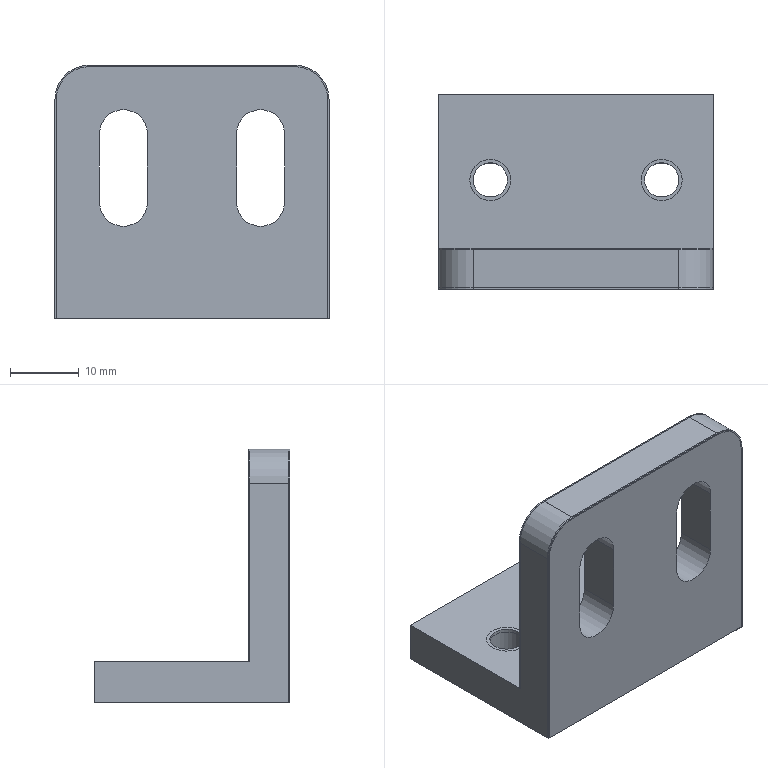Part | 2 solids | 52 faces | box 40 x 28.5 x 37 mm | volume 25348 mm3 | plane 30 | cylinder 16 | cone 6 | commonest cylinder face diameters 7 x8 5 x4 10 x4
STEP:
#1=CARTESIAN_POINT('',(37.,28.5,6.));
#2=VERTEX_POINT('',#1);
#3=CARTESIAN_POINT('',(-3.,28.5,6.));
#4=VERTEX_POINT('',#3);
#5=CARTESIAN_POINT('',(43.57,28.5,6.));
#6=DIRECTION('',(-1.,0.,0.));
#7=VECTOR('',#6,1000.);
#8=LINE('',#5,#7);
#9=EDGE_CURVE('',#2,#4,#8,.T.);
#10=ORIENTED_EDGE('',*,*,#9,.F.);
#11=CARTESIAN_POINT('',(37.,28.5,0.));
#12=VERTEX_POINT('',#11);
#13=CARTESIAN_POINT('',(37.,28.5,0.));
#14=DIRECTION('',(0.,0.,1.));
#15=VECTOR('',#14,1000.);
#16=LINE('',#13,#15);
#17=EDGE_CURVE('',#12,#2,#16,.T.);
#18=ORIENTED_EDGE('',*,*,#17,.F.);
#19=CARTESIAN_POINT('',(-3.,28.5,0.));
#20=VERTEX_POINT('',#19);
#21=CARTESIAN_POINT('',(18.5,28.5,0.));
#22=DIRECTION('',(-1.,0.,0.));
#23=VECTOR('',#22,1000.);
#24=LINE('',#21,#23);
#25=EDGE_CURVE('',#12,#20,#24,.T.);
#26=ORIENTED_EDGE('',*,*,#25,.T.);
#27=CARTESIAN_POINT('',(-3.,28.5,0.));
#28=DIRECTION('',(0.,0.,1.));
#29=VECTOR('',#28,1000.);
#30=LINE('',#27,#29);
#31=EDGE_CURVE('',#20,#4,#30,.T.);
#32=ORIENTED_EDGE('',*,*,#31,.T.);
#33=EDGE_LOOP('',(#10,#18,#26,#32));
#34=FACE_BOUND('',#33,.T.);
#35=CARTESIAN_POINT('',(18.5,28.5,0.));
#36=DIRECTION('',(0.,1.,0.));
#37=DIRECTION('',(0.,0.,1.));
#38=AXIS2_PLACEMENT_3D('',#35,#36,#37);
#39=PLANE('',#38);
#40=ADVANCED_FACE('',(#34),#39,.T.);
#41=CARTESIAN_POINT('',(2.,6.,37.));
#42=VERTEX_POINT('',#41);
#43=CARTESIAN_POINT('',(32.,6.,37.));
#44=VERTEX_POINT('',#43);
#45=CARTESIAN_POINT('',(43.57,6.,37.));
#46=DIRECTION('',(-1.,0.,0.));
#47=VECTOR('',#46,1000.);
#48=LINE('',#45,#47);
#49=EDGE_CURVE('',#42,#44,#48,.F.);
#50=ORIENTED_EDGE('',*,*,#49,.F.);
#51=CARTESIAN_POINT('',(2.,0.,37.));
#52=VERTEX_POINT('',#51);
#53=CARTESIAN_POINT('',(2.,14.25,37.));
#54=DIRECTION('',(0.,1.,0.));
#55=VECTOR('',#54,1000.);
#56=LINE('',#53,#55);
#57=EDGE_CURVE('',#42,#52,#56,.F.);
#58=ORIENTED_EDGE('',*,*,#57,.T.);
#59=CARTESIAN_POINT('',(32.,0.,37.));
#60=VERTEX_POINT('',#59);
#61=CARTESIAN_POINT('',(18.5,0.,37.));
#62=DIRECTION('',(-1.,0.,0.));
#63=VECTOR('',#62,1000.);
#64=LINE('',#61,#63);
#65=EDGE_CURVE('',#60,#52,#64,.T.);
#66=ORIENTED_EDGE('',*,*,#65,.F.);
#67=CARTESIAN_POINT('',(32.,14.25,37.));
#68=DIRECTION('',(0.,-1.,0.));
#69=VECTOR('',#68,1000.);
#70=LINE('',#67,#69);
#71=EDGE_CURVE('',#60,#44,#70,.F.);
#72=ORIENTED_EDGE('',*,*,#71,.T.);
#73=EDGE_LOOP('',(#50,#58,#66,#72));
#74=FACE_BOUND('',#73,.T.);
#75=CARTESIAN_POINT('',(18.5,14.25,37.));
#76=DIRECTION('',(0.,0.,1.));
#77=DIRECTION('',(1.,0.,0.));
#78=AXIS2_PLACEMENT_3D('',#75,#76,#77);
#79=PLANE('',#78);
#80=ADVANCED_FACE('',(#74),#79,.T.);
#81=CARTESIAN_POINT('',(10.5,0.,17.));
#82=VERTEX_POINT('',#81);
#83=CARTESIAN_POINT('',(10.5,0.,27.));
#84=VERTEX_POINT('',#83);
#85=CARTESIAN_POINT('',(10.5,0.,-0.5));
#86=DIRECTION('',(0.,0.,1.));
#87=VECTOR('',#86,1000.);
#88=LINE('',#85,#87);
#89=EDGE_CURVE('',#82,#84,#88,.T.);
#90=ORIENTED_EDGE('',*,*,#89,.F.);
#91=CARTESIAN_POINT('',(3.5,0.,17.));
#92=VERTEX_POINT('',#91);
#93=CARTESIAN_POINT('',(7.,0.,17.));
#94=DIRECTION('',(0.,-1.,0.));
#95=DIRECTION('',(0.,0.,-1.));
#96=AXIS2_PLACEMENT_3D('',#93,#94,#95);
#97=CIRCLE('',#96,3.5);
#98=EDGE_CURVE('',#92,#82,#97,.T.);
#99=ORIENTED_EDGE('',*,*,#98,.F.);
#100=CARTESIAN_POINT('',(3.5,0.,27.));
#101=VERTEX_POINT('',#100);
#102=CARTESIAN_POINT('',(3.5,0.,-0.5));
#103=DIRECTION('',(0.,0.,-1.));
#104=VECTOR('',#103,1000.);
#105=LINE('',#102,#104);
#106=EDGE_CURVE('',#101,#92,#105,.T.);
#107=ORIENTED_EDGE('',*,*,#106,.F.);
#108=CARTESIAN_POINT('',(7.,0.,27.));
#109=DIRECTION('',(0.,-1.,0.));
#110=DIRECTION('',(0.,0.,-1.));
#111=AXIS2_PLACEMENT_3D('',#108,#109,#110);
#112=CIRCLE('',#111,3.5);
#113=EDGE_CURVE('',#84,#101,#112,.T.);
#114=ORIENTED_EDGE('',*,*,#113,.F.);
#115=EDGE_LOOP('',(#90,#99,#107,#114));
#116=FACE_BOUND('',#115,.T.);
#117=CARTESIAN_POINT('',(30.5,0.,17.));
#118=VERTEX_POINT('',#117);
#119=CARTESIAN_POINT('',(30.5,0.,27.));
#120=VERTEX_POINT('',#119);
#121=CARTESIAN_POINT('',(30.5,0.,-0.5));
#122=DIRECTION('',(0.,0.,1.));
#123=VECTOR('',#122,1000.);
#124=LINE('',#121,#123);
#125=EDGE_CURVE('',#118,#120,#124,.T.);
#126=ORIENTED_EDGE('',*,*,#125,.F.);
#127=CARTESIAN_POINT('',(23.5,0.,17.));
#128=VERTEX_POINT('',#127);
#129=CARTESIAN_POINT('',(27.,0.,17.));
#130=DIRECTION('',(0.,-1.,0.));
#131=DIRECTION('',(0.,0.,-1.));
#132=AXIS2_PLACEMENT_3D('',#129,#130,#131);
#133=CIRCLE('',#132,3.5);
#134=EDGE_CURVE('',#128,#118,#133,.T.);
#135=ORIENTED_EDGE('',*,*,#134,.F.);
#136=CARTESIAN_POINT('',(23.5,0.,27.));
#137=VERTEX_POINT('',#136);
#138=CARTESIAN_POINT('',(23.5,0.,-0.5));
#139=DIRECTION('',(0.,0.,-1.));
#140=VECTOR('',#139,1000.);
#141=LINE('',#138,#140);
#142=EDGE_CURVE('',#137,#128,#141,.T.);
#143=ORIENTED_EDGE('',*,*,#142,.F.);
#144=CARTESIAN_POINT('',(27.,0.,27.));
#145=DIRECTION('',(0.,-1.,0.));
#146=DIRECTION('',(0.,0.,-1.));
#147=AXIS2_PLACEMENT_3D('',#144,#145,#146);
#148=CIRCLE('',#147,3.5);
#149=EDGE_CURVE('',#120,#137,#148,.T.);
#150=ORIENTED_EDGE('',*,*,#149,.F.);
#151=EDGE_LOOP('',(#126,#135,#143,#150));
#152=FACE_BOUND('',#151,.T.);
#153=ORIENTED_EDGE('',*,*,#65,.T.);
#154=CARTESIAN_POINT('',(-3.,0.,32.));
#155=VERTEX_POINT('',#154);
#156=CARTESIAN_POINT('',(2.,0.,32.));
#157=DIRECTION('',(0.,-1.,0.));
#158=DIRECTION('',(0.,0.,-1.));
#159=AXIS2_PLACEMENT_3D('',#156,#157,#158);
#160=CIRCLE('',#159,5.);
#161=EDGE_CURVE('',#52,#155,#160,.T.);
#162=ORIENTED_EDGE('',*,*,#161,.T.);
#163=CARTESIAN_POINT('',(-3.,0.,0.));
#164=VERTEX_POINT('',#163);
#165=CARTESIAN_POINT('',(-3.,0.,0.));
#166=DIRECTION('',(0.,0.,1.));
#167=VECTOR('',#166,1000.);
#168=LINE('',#165,#167);
#169=EDGE_CURVE('',#164,#155,#168,.T.);
#170=ORIENTED_EDGE('',*,*,#169,.F.);
#171=CARTESIAN_POINT('',(37.,0.,0.));
#172=VERTEX_POINT('',#171);
#173=CARTESIAN_POINT('',(18.5,0.,0.));
#174=DIRECTION('',(1.,0.,0.));
#175=VECTOR('',#174,1000.);
#176=LINE('',#173,#175);
#177=EDGE_CURVE('',#164,#172,#176,.T.);
#178=ORIENTED_EDGE('',*,*,#177,.T.);
#179=CARTESIAN_POINT('',(37.,0.,32.));
#180=VERTEX_POINT('',#179);
#181=CARTESIAN_POINT('',(37.,0.,0.));
#182=DIRECTION('',(0.,0.,1.));
#183=VECTOR('',#182,1000.);
#184=LINE('',#181,#183);
#185=EDGE_CURVE('',#172,#180,#184,.T.);
#186=ORIENTED_EDGE('',*,*,#185,.T.);
#187=CARTESIAN_POINT('',(32.,0.,32.));
#188=DIRECTION('',(0.,-1.,0.));
#189=DIRECTION('',(0.,0.,-1.));
#190=AXIS2_PLACEMENT_3D('',#187,#188,#189);
#191=CIRCLE('',#190,5.);
#192=EDGE_CURVE('',#180,#60,#191,.T.);
#193=ORIENTED_EDGE('',*,*,#192,.T.);
#194=EDGE_LOOP('',(#153,#162,#170,#178,#186,#193));
#195=FACE_BOUND('',#194,.T.);
#196=CARTESIAN_POINT('',(18.5,0.,0.));
#197=DIRECTION('',(0.,-1.,0.));
#198=DIRECTION('',(0.,0.,-1.));
#199=AXIS2_PLACEMENT_3D('',#196,#197,#198);
#200=PLANE('',#199);
#201=ADVANCED_FACE('',(#116,#152,#195),#200,.T.);
#202=ORIENTED_EDGE('',*,*,#169,.T.);
#203=CARTESIAN_POINT('',(-3.,6.,32.));
#204=VERTEX_POINT('',#203);
#205=CARTESIAN_POINT('',(-3.,14.25,32.));
#206=DIRECTION('',(0.,1.,0.));
#207=VECTOR('',#206,1000.);
#208=LINE('',#205,#207);
#209=EDGE_CURVE('',#155,#204,#208,.T.);
#210=ORIENTED_EDGE('',*,*,#209,.T.);
#211=CARTESIAN_POINT('',(-3.,6.,6.));
#212=VERTEX_POINT('',#211);
#213=CARTESIAN_POINT('',(-3.,6.,0.));
#214=DIRECTION('',(0.,0.,1.));
#215=VECTOR('',#214,1000.);
#216=LINE('',#213,#215);
#217=EDGE_CURVE('',#212,#204,#216,.T.);
#218=ORIENTED_EDGE('',*,*,#217,.F.);
#219=CARTESIAN_POINT('',(-3.,14.25,6.));
#220=DIRECTION('',(0.,-1.,0.));
#221=VECTOR('',#220,1000.);
#222=LINE('',#219,#221);
#223=EDGE_CURVE('',#4,#212,#222,.T.);
#224=ORIENTED_EDGE('',*,*,#223,.F.);
#225=ORIENTED_EDGE('',*,*,#31,.F.);
#226=CARTESIAN_POINT('',(-3.,14.25,0.));
#227=DIRECTION('',(0.,-1.,0.));
#228=VECTOR('',#227,1000.);
#229=LINE('',#226,#228);
#230=EDGE_CURVE('',#20,#164,#229,.T.);
#231=ORIENTED_EDGE('',*,*,#230,.T.);
#232=EDGE_LOOP('',(#202,#210,#218,#224,#225,#231));
#233=FACE_BOUND('',#232,.T.);
#234=CARTESIAN_POINT('',(-3.,14.25,0.));
#235=DIRECTION('',(-1.,0.,0.));
#236=DIRECTION('',(0.,0.,1.));
#237=AXIS2_PLACEMENT_3D('',#234,#235,#236);
#238=PLANE('',#237);
#239=ADVANCED_FACE('',(#233),#238,.T.);
#240=CARTESIAN_POINT('',(32.,16.,0.));
#241=VERTEX_POINT('',#240);
#242=CARTESIAN_POINT('',(29.5,16.,0.));
#243=DIRECTION('',(0.,0.,1.));
#244=DIRECTION('',(1.,0.,0.));
#245=AXIS2_PLACEMENT_3D('',#242,#243,#244);
#246=CIRCLE('',#245,2.5);
#247=EDGE_CURVE('',#241,#241,#246,.T.);
#248=ORIENTED_EDGE('',*,*,#247,.T.);
#249=EDGE_LOOP('',(#248));
#250=FACE_BOUND('',#249,.T.);
#251=CARTESIAN_POINT('',(7.,16.,0.));
#252=VERTEX_POINT('',#251);
#253=CARTESIAN_POINT('',(4.5,16.,0.));
#254=DIRECTION('',(0.,0.,1.));
#255=DIRECTION('',(1.,0.,0.));
#256=AXIS2_PLACEMENT_3D('',#253,#254,#255);
#257=CIRCLE('',#256,2.5);
#258=EDGE_CURVE('',#252,#252,#257,.T.);
#259=ORIENTED_EDGE('',*,*,#258,.T.);
#260=EDGE_LOOP('',(#259));
#261=FACE_BOUND('',#260,.T.);
#262=CARTESIAN_POINT('',(37.,14.25,0.));
#263=DIRECTION('',(0.,1.,0.));
#264=VECTOR('',#263,1000.);
#265=LINE('',#262,#264);
#266=EDGE_CURVE('',#172,#12,#265,.T.);
#267=ORIENTED_EDGE('',*,*,#266,.F.);
#268=ORIENTED_EDGE('',*,*,#177,.F.);
#269=ORIENTED_EDGE('',*,*,#230,.F.);
#270=ORIENTED_EDGE('',*,*,#25,.F.);
#271=EDGE_LOOP('',(#267,#268,#269,#270));
#272=FACE_BOUND('',#271,.T.);
#273=CARTESIAN_POINT('',(18.5,14.25,0.));
#274=DIRECTION('',(0.,0.,-1.));
#275=DIRECTION('',(-1.,0.,0.));
#276=AXIS2_PLACEMENT_3D('',#273,#274,#275);
#277=PLANE('',#276);
#278=ADVANCED_FACE('',(#250,#261,#272),#277,.T.);
#279=CARTESIAN_POINT('',(37.,6.,32.));
#280=VERTEX_POINT('',#279);
#281=CARTESIAN_POINT('',(37.,6.,6.));
#282=VERTEX_POINT('',#281);
#283=CARTESIAN_POINT('',(37.,6.,0.));
#284=DIRECTION('',(0.,0.,-1.));
#285=VECTOR('',#284,1000.);
#286=LINE('',#283,#285);
#287=EDGE_CURVE('',#280,#282,#286,.T.);
#288=ORIENTED_EDGE('',*,*,#287,.F.);
#289=CARTESIAN_POINT('',(37.,14.25,32.));
#290=DIRECTION('',(0.,-1.,0.));
#291=VECTOR('',#290,1000.);
#292=LINE('',#289,#291);
#293=EDGE_CURVE('',#280,#180,#292,.T.);
#294=ORIENTED_EDGE('',*,*,#293,.T.);
#295=ORIENTED_EDGE('',*,*,#185,.F.);
#296=ORIENTED_EDGE('',*,*,#266,.T.);
#297=ORIENTED_EDGE('',*,*,#17,.T.);
#298=CARTESIAN_POINT('',(37.,14.25,6.));
#299=DIRECTION('',(0.,1.,0.));
#300=VECTOR('',#299,1000.);
#301=LINE('',#298,#300);
#302=EDGE_CURVE('',#282,#2,#301,.T.);
#303=ORIENTED_EDGE('',*,*,#302,.F.);
#304=EDGE_LOOP('',(#288,#294,#295,#296,#297,#303));
#305=FACE_BOUND('',#304,.T.);
#306=CARTESIAN_POINT('',(37.,14.25,0.));
#307=DIRECTION('',(1.,0.,0.));
#308=DIRECTION('',(0.,0.,-1.));
#309=AXIS2_PLACEMENT_3D('',#306,#307,#308);
#310=PLANE('',#309);
#311=ADVANCED_FACE('',(#305),#310,.T.);
#312=CARTESIAN_POINT('',(27.,16.,6.));
#313=VERTEX_POINT('',#312);
#314=CARTESIAN_POINT('',(29.5,16.,6.));
#315=DIRECTION('',(0.,0.,-1.));
#316=DIRECTION('',(-1.,0.,0.));
#317=AXIS2_PLACEMENT_3D('',#314,#315,#316);
#318=CIRCLE('',#317,2.5);
#319=EDGE_CURVE('',#313,#313,#318,.T.);
#320=ORIENTED_EDGE('',*,*,#319,.T.);
#321=EDGE_LOOP('',(#320));
#322=FACE_BOUND('',#321,.T.);
#323=CARTESIAN_POINT('',(2.,16.,6.));
#324=VERTEX_POINT('',#323);
#325=CARTESIAN_POINT('',(4.5,16.,6.));
#326=DIRECTION('',(0.,0.,-1.));
#327=DIRECTION('',(-1.,0.,0.));
#328=AXIS2_PLACEMENT_3D('',#325,#326,#327);
#329=CIRCLE('',#328,2.5);
#330=EDGE_CURVE('',#324,#324,#329,.T.);
#331=ORIENTED_EDGE('',*,*,#330,.T.);
#332=EDGE_LOOP('',(#331));
#333=FACE_BOUND('',#332,.T.);
#334=ORIENTED_EDGE('',*,*,#223,.T.);
#335=CARTESIAN_POINT('',(43.57,6.,6.));
#336=DIRECTION('',(-1.,0.,0.));
#337=VECTOR('',#336,1000.);
#338=LINE('',#335,#337);
#339=EDGE_CURVE('',#212,#282,#338,.F.);
#340=ORIENTED_EDGE('',*,*,#339,.T.);
#341=ORIENTED_EDGE('',*,*,#302,.T.);
#342=ORIENTED_EDGE('',*,*,#9,.T.);
#343=EDGE_LOOP('',(#334,#340,#341,#342));
#344=FACE_BOUND('',#343,.T.);
#345=CARTESIAN_POINT('',(43.57,28.5,6.));
#346=DIRECTION('',(0.,0.,-1.));
#347=DIRECTION('',(-1.,0.,0.));
#348=AXIS2_PLACEMENT_3D('',#345,#346,#347);
#349=PLANE('',#348);
#350=ADVANCED_FACE('',(#322,#333,#344),#349,.F.);
#351=CARTESIAN_POINT('',(10.5,6.,17.));
#352=VERTEX_POINT('',#351);
#353=CARTESIAN_POINT('',(3.5,6.,17.));
#354=VERTEX_POINT('',#353);
#355=CARTESIAN_POINT('',(7.,6.,17.));
#356=DIRECTION('',(0.,1.,0.));
#357=DIRECTION('',(0.,0.,1.));
#358=AXIS2_PLACEMENT_3D('',#355,#356,#357);
#359=CIRCLE('',#358,3.5);
#360=EDGE_CURVE('',#352,#354,#359,.T.);
#361=ORIENTED_EDGE('',*,*,#360,.F.);
#362=CARTESIAN_POINT('',(10.5,6.,27.));
#363=VERTEX_POINT('',#362);
#364=CARTESIAN_POINT('',(10.5,6.,22.));
#365=DIRECTION('',(0.,0.,1.));
#366=VECTOR('',#365,1000.);
#367=LINE('',#364,#366);
#368=EDGE_CURVE('',#352,#363,#367,.T.);
#369=ORIENTED_EDGE('',*,*,#368,.T.);
#370=CARTESIAN_POINT('',(3.5,6.,27.));
#371=VERTEX_POINT('',#370);
#372=CARTESIAN_POINT('',(7.,6.,27.));
#373=DIRECTION('',(0.,1.,0.));
#374=DIRECTION('',(0.,0.,1.));
#375=AXIS2_PLACEMENT_3D('',#372,#373,#374);
#376=CIRCLE('',#375,3.5);
#377=EDGE_CURVE('',#371,#363,#376,.T.);
#378=ORIENTED_EDGE('',*,*,#377,.F.);
#379=CARTESIAN_POINT('',(3.5,6.,22.));
#380=DIRECTION('',(0.,0.,1.));
#381=VECTOR('',#380,1000.);
#382=LINE('',#379,#381);
#383=EDGE_CURVE('',#354,#371,#382,.T.);
#384=ORIENTED_EDGE('',*,*,#383,.F.);
#385=EDGE_LOOP('',(#361,#369,#378,#384));
#386=FACE_BOUND('',#385,.T.);
#387=CARTESIAN_POINT('',(30.5,6.,17.));
#388=VERTEX_POINT('',#387);
#389=CARTESIAN_POINT('',(23.5,6.,17.));
#390=VERTEX_POINT('',#389);
#391=CARTESIAN_POINT('',(27.,6.,17.));
#392=DIRECTION('',(0.,1.,0.));
#393=DIRECTION('',(0.,0.,1.));
#394=AXIS2_PLACEMENT_3D('',#391,#392,#393);
#395=CIRCLE('',#394,3.5);
#396=EDGE_CURVE('',#388,#390,#395,.T.);
#397=ORIENTED_EDGE('',*,*,#396,.F.);
#398=CARTESIAN_POINT('',(30.5,6.,27.));
#399=VERTEX_POINT('',#398);
#400=CARTESIAN_POINT('',(30.5,6.,22.));
#401=DIRECTION('',(0.,0.,1.));
#402=VECTOR('',#401,1000.);
#403=LINE('',#400,#402);
#404=EDGE_CURVE('',#388,#399,#403,.T.);
#405=ORIENTED_EDGE('',*,*,#404,.T.);
#406=CARTESIAN_POINT('',(23.5,6.,27.));
#407=VERTEX_POINT('',#406);
#408=CARTESIAN_POINT('',(27.,6.,27.));
#409=DIRECTION('',(0.,1.,0.));
#410=DIRECTION('',(0.,0.,1.));
#411=AXIS2_PLACEMENT_3D('',#408,#409,#410);
#412=CIRCLE('',#411,3.5);
#413=EDGE_CURVE('',#407,#399,#412,.T.);
#414=ORIENTED_EDGE('',*,*,#413,.F.);
#415=CARTESIAN_POINT('',(23.5,6.,22.));
#416=DIRECTION('',(0.,0.,1.));
#417=VECTOR('',#416,1000.);
#418=LINE('',#415,#417);
#419=EDGE_CURVE('',#390,#407,#418,.T.);
#420=ORIENTED_EDGE('',*,*,#419,.F.);
#421=EDGE_LOOP('',(#397,#405,#414,#420));
#422=FACE_BOUND('',#421,.T.);
#423=ORIENTED_EDGE('',*,*,#217,.T.);
#424=CARTESIAN_POINT('',(2.,6.,32.));
#425=DIRECTION('',(0.,-1.,0.));
#426=DIRECTION('',(0.,0.,-1.));
#427=AXIS2_PLACEMENT_3D('',#424,#425,#426);
#428=CIRCLE('',#427,5.);
#429=EDGE_CURVE('',#204,#42,#428,.F.);
#430=ORIENTED_EDGE('',*,*,#429,.T.);
#431=ORIENTED_EDGE('',*,*,#49,.T.);
#432=CARTESIAN_POINT('',(32.,6.,32.));
#433=DIRECTION('',(0.,-1.,0.));
#434=DIRECTION('',(0.,0.,-1.));
#435=AXIS2_PLACEMENT_3D('',#432,#433,#434);
#436=CIRCLE('',#435,5.);
#437=EDGE_CURVE('',#44,#280,#436,.F.);
#438=ORIENTED_EDGE('',*,*,#437,.T.);
#439=ORIENTED_EDGE('',*,*,#287,.T.);
#440=ORIENTED_EDGE('',*,*,#339,.F.);
#441=EDGE_LOOP('',(#423,#430,#431,#438,#439,#440));
#442=FACE_BOUND('',#441,.T.);
#443=CARTESIAN_POINT('',(43.57,6.,37.));
#444=DIRECTION('',(0.,-1.,0.));
#445=DIRECTION('',(0.,0.,-1.));
#446=AXIS2_PLACEMENT_3D('',#443,#444,#445);
#447=PLANE('',#446);
#448=ADVANCED_FACE('',(#386,#422,#442),#447,.F.);
#449=ORIENTED_EDGE('',*,*,#125,.T.);
#450=CARTESIAN_POINT('',(30.5,6.,27.));
#451=DIRECTION('',(0.,1.,0.));
#452=VECTOR('',#451,1000.);
#453=LINE('',#450,#452);
#454=EDGE_CURVE('',#399,#120,#453,.F.);
#455=ORIENTED_EDGE('',*,*,#454,.F.);
#456=ORIENTED_EDGE('',*,*,#404,.F.);
#457=CARTESIAN_POINT('',(30.5,6.,17.));
#458=DIRECTION('',(0.,1.,0.));
#459=VECTOR('',#458,1000.);
#460=LINE('',#457,#459);
#461=EDGE_CURVE('',#388,#118,#460,.F.);
#462=ORIENTED_EDGE('',*,*,#461,.T.);
#463=EDGE_LOOP('',(#449,#455,#456,#462));
#464=FACE_BOUND('',#463,.T.);
#465=CARTESIAN_POINT('',(30.5,6.,22.));
#466=DIRECTION('',(1.,0.,0.));
#467=DIRECTION('',(0.,0.,-1.));
#468=AXIS2_PLACEMENT_3D('',#465,#466,#467);
#469=PLANE('',#468);
#470=ADVANCED_FACE('',(#464),#469,.F.);
#471=ORIENTED_EDGE('',*,*,#134,.T.);
#472=ORIENTED_EDGE('',*,*,#461,.F.);
#473=ORIENTED_EDGE('',*,*,#396,.T.);
#474=CARTESIAN_POINT('',(23.5,6.,17.));
#475=DIRECTION('',(0.,1.,0.));
#476=VECTOR('',#475,1000.);
#477=LINE('',#474,#476);
#478=EDGE_CURVE('',#390,#128,#477,.F.);
#479=ORIENTED_EDGE('',*,*,#478,.T.);
#480=EDGE_LOOP('',(#471,#472,#473,#479));
#481=FACE_BOUND('',#480,.T.);
#482=CARTESIAN_POINT('',(27.,6.,17.));
#483=DIRECTION('',(0.,1.,0.));
#484=DIRECTION('',(0.,0.,1.));
#485=AXIS2_PLACEMENT_3D('',#482,#483,#484);
#486=CYLINDRICAL_SURFACE('',#485,3.5);
#487=ADVANCED_FACE('',(#481),#486,.F.);
#488=ORIENTED_EDGE('',*,*,#142,.T.);
#489=ORIENTED_EDGE('',*,*,#478,.F.);
#490=ORIENTED_EDGE('',*,*,#419,.T.);
#491=CARTESIAN_POINT('',(23.5,6.,27.));
#492=DIRECTION('',(0.,1.,0.));
#493=VECTOR('',#492,1000.);
#494=LINE('',#491,#493);
#495=EDGE_CURVE('',#407,#137,#494,.F.);
#496=ORIENTED_EDGE('',*,*,#495,.T.);
#497=EDGE_LOOP('',(#488,#489,#490,#496));
#498=FACE_BOUND('',#497,.T.);
#499=CARTESIAN_POINT('',(23.5,6.,22.));
#500=DIRECTION('',(-1.,0.,0.));
#501=DIRECTION('',(0.,0.,1.));
#502=AXIS2_PLACEMENT_3D('',#499,#500,#501);
#503=PLANE('',#502);
#504=ADVANCED_FACE('',(#498),#503,.F.);
#505=ORIENTED_EDGE('',*,*,#149,.T.);
#506=ORIENTED_EDGE('',*,*,#495,.F.);
#507=ORIENTED_EDGE('',*,*,#413,.T.);
#508=ORIENTED_EDGE('',*,*,#454,.T.);
#509=EDGE_LOOP('',(#505,#506,#507,#508));
#510=FACE_BOUND('',#509,.T.);
#511=CARTESIAN_POINT('',(27.,6.,27.));
#512=DIRECTION('',(0.,1.,0.));
#513=DIRECTION('',(0.,0.,1.));
#514=AXIS2_PLACEMENT_3D('',#511,#512,#513);
#515=CYLINDRICAL_SURFACE('',#514,3.5);
#516=ADVANCED_FACE('',(#510),#515,.F.);
#517=ORIENTED_EDGE('',*,*,#89,.T.);
#518=CARTESIAN_POINT('',(10.5,6.,27.));
#519=DIRECTION('',(0.,1.,0.));
#520=VECTOR('',#519,1000.);
#521=LINE('',#518,#520);
#522=EDGE_CURVE('',#84,#363,#521,.T.);
#523=ORIENTED_EDGE('',*,*,#522,.T.);
#524=ORIENTED_EDGE('',*,*,#368,.F.);
#525=CARTESIAN_POINT('',(10.5,6.,17.));
#526=DIRECTION('',(0.,1.,0.));
#527=VECTOR('',#526,1000.);
#528=LINE('',#525,#527);
#529=EDGE_CURVE('',#82,#352,#528,.T.);
#530=ORIENTED_EDGE('',*,*,#529,.F.);
#531=EDGE_LOOP('',(#517,#523,#524,#530));
#532=FACE_BOUND('',#531,.T.);
#533=CARTESIAN_POINT('',(10.5,6.,22.));
#534=DIRECTION('',(1.,0.,0.));
#535=DIRECTION('',(0.,0.,-1.));
#536=AXIS2_PLACEMENT_3D('',#533,#534,#535);
#537=PLANE('',#536);
#538=ADVANCED_FACE('',(#532),#537,.F.);
#539=ORIENTED_EDGE('',*,*,#98,.T.);
#540=ORIENTED_EDGE('',*,*,#529,.T.);
#541=ORIENTED_EDGE('',*,*,#360,.T.);
#542=CARTESIAN_POINT('',(3.5,6.,17.));
#543=DIRECTION('',(0.,1.,0.));
#544=VECTOR('',#543,1000.);
#545=LINE('',#542,#544);
#546=EDGE_CURVE('',#92,#354,#545,.T.);
#547=ORIENTED_EDGE('',*,*,#546,.F.);
#548=EDGE_LOOP('',(#539,#540,#541,#547));
#549=FACE_BOUND('',#548,.T.);
#550=CARTESIAN_POINT('',(7.,6.,17.));
#551=DIRECTION('',(0.,1.,0.));
#552=DIRECTION('',(0.,0.,1.));
#553=AXIS2_PLACEMENT_3D('',#550,#551,#552);
#554=CYLINDRICAL_SURFACE('',#553,3.5);
#555=ADVANCED_FACE('',(#549),#554,.F.);
#556=ORIENTED_EDGE('',*,*,#106,.T.);
#557=ORIENTED_EDGE('',*,*,#546,.T.);
#558=ORIENTED_EDGE('',*,*,#383,.T.);
#559=CARTESIAN_POINT('',(3.5,6.,27.));
#560=DIRECTION('',(0.,1.,0.));
#561=VECTOR('',#560,1000.);
#562=LINE('',#559,#561);
#563=EDGE_CURVE('',#101,#371,#562,.T.);
#564=ORIENTED_EDGE('',*,*,#563,.F.);
#565=EDGE_LOOP('',(#556,#557,#558,#564));
#566=FACE_BOUND('',#565,.T.);
#567=CARTESIAN_POINT('',(3.5,6.,22.));
#568=DIRECTION('',(-1.,0.,0.));
#569=DIRECTION('',(0.,0.,1.));
#570=AXIS2_PLACEMENT_3D('',#567,#568,#569);
#571=PLANE('',#570);
#572=ADVANCED_FACE('',(#566),#571,.F.);
#573=ORIENTED_EDGE('',*,*,#113,.T.);
#574=ORIENTED_EDGE('',*,*,#563,.T.);
#575=ORIENTED_EDGE('',*,*,#377,.T.);
#576=ORIENTED_EDGE('',*,*,#522,.F.);
#577=EDGE_LOOP('',(#573,#574,#575,#576));
#578=FACE_BOUND('',#577,.T.);
#579=CARTESIAN_POINT('',(7.,6.,27.));
#580=DIRECTION('',(0.,1.,0.));
#581=DIRECTION('',(0.,0.,1.));
#582=AXIS2_PLACEMENT_3D('',#579,#580,#581);
#583=CYLINDRICAL_SURFACE('',#582,3.5);
#584=ADVANCED_FACE('',(#578),#583,.F.);
#585=ORIENTED_EDGE('',*,*,#161,.F.);
#586=ORIENTED_EDGE('',*,*,#57,.F.);
#587=ORIENTED_EDGE('',*,*,#429,.F.);
#588=ORIENTED_EDGE('',*,*,#209,.F.);
#589=EDGE_LOOP('',(#585,#586,#587,#588));
#590=FACE_BOUND('',#589,.T.);
#591=CARTESIAN_POINT('',(2.,14.25,32.));
#592=DIRECTION('',(0.,1.,0.));
#593=DIRECTION('',(0.,0.,1.));
#594=AXIS2_PLACEMENT_3D('',#591,#592,#593);
#595=CYLINDRICAL_SURFACE('',#594,5.);
#596=ADVANCED_FACE('',(#590),#595,.T.);
#597=ORIENTED_EDGE('',*,*,#437,.F.);
#598=ORIENTED_EDGE('',*,*,#71,.F.);
#599=ORIENTED_EDGE('',*,*,#192,.F.);
#600=ORIENTED_EDGE('',*,*,#293,.F.);
#601=EDGE_LOOP('',(#597,#598,#599,#600));
#602=FACE_BOUND('',#601,.T.);
#603=CARTESIAN_POINT('',(32.,14.25,32.));
#604=DIRECTION('',(0.,-1.,0.));
#605=DIRECTION('',(0.,0.,-1.));
#606=AXIS2_PLACEMENT_3D('',#603,#604,#605);
#607=CYLINDRICAL_SURFACE('',#606,5.);
#608=ADVANCED_FACE('',(#602),#607,.T.);
#609=ORIENTED_EDGE('',*,*,#258,.F.);
#610=EDGE_LOOP('',(#609));
#611=FACE_BOUND('',#610,.T.);
#612=ORIENTED_EDGE('',*,*,#330,.F.);
#613=EDGE_LOOP('',(#612));
#614=FACE_BOUND('',#613,.T.);
#615=CARTESIAN_POINT('',(4.5,16.,0.));
#616=DIRECTION('',(0.,0.,1.));
#617=DIRECTION('',(1.,0.,0.));
#618=AXIS2_PLACEMENT_3D('',#615,#616,#617);
#619=CYLINDRICAL_SURFACE('',#618,2.5);
#620=ADVANCED_FACE('',(#611,#614),#619,.F.);
#621=ORIENTED_EDGE('',*,*,#247,.F.);
#622=EDGE_LOOP('',(#621));
#623=FACE_BOUND('',#622,.T.);
#624=ORIENTED_EDGE('',*,*,#319,.F.);
#625=EDGE_LOOP('',(#624));
#626=FACE_BOUND('',#625,.T.);
#627=CARTESIAN_POINT('',(29.5,16.,0.));
#628=DIRECTION('',(0.,0.,1.));
#629=DIRECTION('',(1.,0.,0.));
#630=AXIS2_PLACEMENT_3D('',#627,#628,#629);
#631=CYLINDRICAL_SURFACE('',#630,2.5);
#632=ADVANCED_FACE('',(#623,#626),#631,.F.);
#633=CLOSED_SHELL('',(#40,#80,#201,#239,#278,#311,#350,#448,#470,#487,#504,#516,#538,#555,#572,#584,#596,#608,#620,#632));
#634=MANIFOLD_SOLID_BREP('',#633);
#635=CARTESIAN_POINT('',(37.,28.5,6.));
#636=VERTEX_POINT('',#635);
#637=CARTESIAN_POINT('',(-3.,28.5,6.));
#638=VERTEX_POINT('',#637);
#639=CARTESIAN_POINT('',(43.57,28.5,6.));
#640=DIRECTION('',(-1.,0.,0.));
#641=VECTOR('',#640,1000.);
#642=LINE('',#639,#641);
#643=EDGE_CURVE('',#636,#638,#642,.T.);
#644=ORIENTED_EDGE('',*,*,#643,.F.);
#645=CARTESIAN_POINT('',(37.,28.5,0.));
#646=VERTEX_POINT('',#645);
#647=CARTESIAN_POINT('',(37.,28.5,0.));
#648=DIRECTION('',(0.,0.,1.));
#649=VECTOR('',#648,1000.);
#650=LINE('',#647,#649);
#651=EDGE_CURVE('',#646,#636,#650,.T.);
#652=ORIENTED_EDGE('',*,*,#651,.F.);
#653=CARTESIAN_POINT('',(-3.,28.5,0.));
#654=VERTEX_POINT('',#653);
#655=CARTESIAN_POINT('',(18.5,28.5,0.));
#656=DIRECTION('',(-1.,0.,0.));
#657=VECTOR('',#656,1000.);
#658=LINE('',#655,#657);
#659=EDGE_CURVE('',#646,#654,#658,.T.);
#660=ORIENTED_EDGE('',*,*,#659,.T.);
#661=CARTESIAN_POINT('',(-3.,28.5,0.));
#662=DIRECTION('',(0.,0.,1.));
#663=VECTOR('',#662,1000.);
#664=LINE('',#661,#663);
#665=EDGE_CURVE('',#654,#638,#664,.T.);
#666=ORIENTED_EDGE('',*,*,#665,.T.);
#667=EDGE_LOOP('',(#644,#652,#660,#666));
#668=FACE_BOUND('',#667,.T.);
#669=CARTESIAN_POINT('',(18.5,28.5,0.));
#670=DIRECTION('',(0.,1.,0.));
#671=DIRECTION('',(0.,0.,1.));
#672=AXIS2_PLACEMENT_3D('',#669,#670,#671);
#673=PLANE('',#672);
#674=ADVANCED_FACE('',(#668),#673,.T.);
#675=CARTESIAN_POINT('',(2.,5.8,37.));
#676=VERTEX_POINT('',#675);
#677=CARTESIAN_POINT('',(2.,0.2,37.));
#678=VERTEX_POINT('',#677);
#679=CARTESIAN_POINT('',(2.,14.25,37.));
#680=DIRECTION('',(0.,1.,0.));
#681=VECTOR('',#680,1000.);
#682=LINE('',#679,#681);
#683=EDGE_CURVE('',#676,#678,#682,.F.);
#684=ORIENTED_EDGE('',*,*,#683,.T.);
#685=CARTESIAN_POINT('',(32.,0.2,37.));
#686=VERTEX_POINT('',#685);
#687=CARTESIAN_POINT('',(18.5,0.2,37.));
#688=DIRECTION('',(1.,0.,0.));
#689=VECTOR('',#688,1000.);
#690=LINE('',#687,#689);
#691=EDGE_CURVE('',#678,#686,#690,.T.);
#692=ORIENTED_EDGE('',*,*,#691,.T.);
#693=CARTESIAN_POINT('',(32.,5.8,37.));
#694=VERTEX_POINT('',#693);
#695=CARTESIAN_POINT('',(32.,14.25,37.));
#696=DIRECTION('',(0.,-1.,0.));
#697=VECTOR('',#696,1000.);
#698=LINE('',#695,#697);
#699=EDGE_CURVE('',#686,#694,#698,.F.);
#700=ORIENTED_EDGE('',*,*,#699,.T.);
#701=CARTESIAN_POINT('',(2.,5.8,37.));
#702=DIRECTION('',(-1.,0.,0.));
#703=VECTOR('',#702,1000.);
#704=LINE('',#701,#703);
#705=EDGE_CURVE('',#694,#676,#704,.T.);
#706=ORIENTED_EDGE('',*,*,#705,.T.);
#707=EDGE_LOOP('',(#684,#692,#700,#706));
#708=FACE_BOUND('',#707,.T.);
#709=CARTESIAN_POINT('',(18.5,14.25,37.));
#710=DIRECTION('',(0.,0.,1.));
#711=DIRECTION('',(1.,0.,0.));
#712=AXIS2_PLACEMENT_3D('',#709,#710,#711);
#713=PLANE('',#712);
#714=ADVANCED_FACE('',(#708),#713,.T.);
#715=CARTESIAN_POINT('',(10.5,0.,17.));
#716=VERTEX_POINT('',#715);
#717=CARTESIAN_POINT('',(10.5,0.,27.));
#718=VERTEX_POINT('',#717);
#719=CARTESIAN_POINT('',(10.5,0.,-0.5));
#720=DIRECTION('',(0.,0.,1.));
#721=VECTOR('',#720,1000.);
#722=LINE('',#719,#721);
#723=EDGE_CURVE('',#716,#718,#722,.T.);
#724=ORIENTED_EDGE('',*,*,#723,.F.);
#725=CARTESIAN_POINT('',(3.5,0.,17.));
#726=VERTEX_POINT('',#725);
#727=CARTESIAN_POINT('',(7.,0.,17.));
#728=DIRECTION('',(0.,-1.,0.));
#729=DIRECTION('',(0.,0.,-1.));
#730=AXIS2_PLACEMENT_3D('',#727,#728,#729);
#731=CIRCLE('',#730,3.5);
#732=EDGE_CURVE('',#726,#716,#731,.T.);
#733=ORIENTED_EDGE('',*,*,#732,.F.);
#734=CARTESIAN_POINT('',(3.5,0.,27.));
#735=VERTEX_POINT('',#734);
#736=CARTESIAN_POINT('',(3.5,0.,-0.5));
#737=DIRECTION('',(0.,0.,-1.));
#738=VECTOR('',#737,1000.);
#739=LINE('',#736,#738);
#740=EDGE_CURVE('',#735,#726,#739,.T.);
#741=ORIENTED_EDGE('',*,*,#740,.F.);
#742=CARTESIAN_POINT('',(7.,0.,27.));
#743=DIRECTION('',(0.,-1.,0.));
#744=DIRECTION('',(0.,0.,-1.));
#745=AXIS2_PLACEMENT_3D('',#742,#743,#744);
#746=CIRCLE('',#745,3.5);
#747=EDGE_CURVE('',#718,#735,#746,.T.);
#748=ORIENTED_EDGE('',*,*,#747,.F.);
#749=EDGE_LOOP('',(#724,#733,#741,#748));
#750=FACE_BOUND('',#749,.T.);
#751=CARTESIAN_POINT('',(30.5,0.,17.));
#752=VERTEX_POINT('',#751);
#753=CARTESIAN_POINT('',(30.5,0.,27.));
#754=VERTEX_POINT('',#753);
#755=CARTESIAN_POINT('',(30.5,0.,-0.5));
#756=DIRECTION('',(0.,0.,1.));
#757=VECTOR('',#756,1000.);
#758=LINE('',#755,#757);
#759=EDGE_CURVE('',#752,#754,#758,.T.);
#760=ORIENTED_EDGE('',*,*,#759,.F.);
#761=CARTESIAN_POINT('',(23.5,0.,17.));
#762=VERTEX_POINT('',#761);
#763=CARTESIAN_POINT('',(27.,0.,17.));
#764=DIRECTION('',(0.,-1.,0.));
#765=DIRECTION('',(0.,0.,-1.));
#766=AXIS2_PLACEMENT_3D('',#763,#764,#765);
#767=CIRCLE('',#766,3.5);
#768=EDGE_CURVE('',#762,#752,#767,.T.);
#769=ORIENTED_EDGE('',*,*,#768,.F.);
#770=CARTESIAN_POINT('',(23.5,0.,27.));
#771=VERTEX_POINT('',#770);
#772=CARTESIAN_POINT('',(23.5,0.,-0.5));
#773=DIRECTION('',(0.,0.,-1.));
#774=VECTOR('',#773,1000.);
#775=LINE('',#772,#774);
#776=EDGE_CURVE('',#771,#762,#775,.T.);
#777=ORIENTED_EDGE('',*,*,#776,.F.);
#778=CARTESIAN_POINT('',(27.,0.,27.));
#779=DIRECTION('',(0.,-1.,0.));
#780=DIRECTION('',(0.,0.,-1.));
#781=AXIS2_PLACEMENT_3D('',#778,#779,#780);
#782=CIRCLE('',#781,3.5);
#783=EDGE_CURVE('',#754,#771,#782,.T.);
#784=ORIENTED_EDGE('',*,*,#783,.F.);
#785=EDGE_LOOP('',(#760,#769,#777,#784));
#786=FACE_BOUND('',#785,.T.);
#787=CARTESIAN_POINT('',(-2.8,0.,0.));
#788=VERTEX_POINT('',#787);
#789=CARTESIAN_POINT('',(36.8,0.,0.));
#790=VERTEX_POINT('',#789);
#791=CARTESIAN_POINT('',(18.5,0.,0.));
#792=DIRECTION('',(1.,0.,0.));
#793=VECTOR('',#792,1000.);
#794=LINE('',#791,#793);
#795=EDGE_CURVE('',#788,#790,#794,.T.);
#796=ORIENTED_EDGE('',*,*,#795,.T.);
#797=CARTESIAN_POINT('',(36.8,0.,32.));
#798=VERTEX_POINT('',#797);
#799=CARTESIAN_POINT('',(36.8,0.,0.));
#800=DIRECTION('',(0.,0.,1.));
#801=VECTOR('',#800,1000.);
#802=LINE('',#799,#801);
#803=EDGE_CURVE('',#790,#798,#802,.T.);
#804=ORIENTED_EDGE('',*,*,#803,.T.);
#805=CARTESIAN_POINT('',(32.,0.,36.8));
#806=VERTEX_POINT('',#805);
#807=CARTESIAN_POINT('',(32.,0.,32.));
#808=DIRECTION('',(0.,-1.,0.));
#809=DIRECTION('',(0.,0.,-1.));
#810=AXIS2_PLACEMENT_3D('',#807,#808,#809);
#811=CIRCLE('',#810,4.8);
#812=EDGE_CURVE('',#798,#806,#811,.T.);
#813=ORIENTED_EDGE('',*,*,#812,.T.);
#814=CARTESIAN_POINT('',(2.,0.,36.8));
#815=VERTEX_POINT('',#814);
#816=CARTESIAN_POINT('',(18.5,0.,36.8));
#817=DIRECTION('',(-1.,0.,0.));
#818=VECTOR('',#817,1000.);
#819=LINE('',#816,#818);
#820=EDGE_CURVE('',#806,#815,#819,.T.);
#821=ORIENTED_EDGE('',*,*,#820,.T.);
#822=CARTESIAN_POINT('',(-2.8,0.,32.));
#823=VERTEX_POINT('',#822);
#824=CARTESIAN_POINT('',(2.,0.,32.));
#825=DIRECTION('',(0.,-1.,0.));
#826=DIRECTION('',(0.,0.,-1.));
#827=AXIS2_PLACEMENT_3D('',#824,#825,#826);
#828=CIRCLE('',#827,4.8);
#829=EDGE_CURVE('',#815,#823,#828,.T.);
#830=ORIENTED_EDGE('',*,*,#829,.T.);
#831=CARTESIAN_POINT('',(-2.8,0.,0.));
#832=DIRECTION('',(0.,0.,-1.));
#833=VECTOR('',#832,1000.);
#834=LINE('',#831,#833);
#835=EDGE_CURVE('',#823,#788,#834,.T.);
#836=ORIENTED_EDGE('',*,*,#835,.T.);
#837=EDGE_LOOP('',(#796,#804,#813,#821,#830,#836));
#838=FACE_BOUND('',#837,.T.);
#839=CARTESIAN_POINT('',(18.5,0.,0.));
#840=DIRECTION('',(0.,-1.,0.));
#841=DIRECTION('',(0.,0.,-1.));
#842=AXIS2_PLACEMENT_3D('',#839,#840,#841);
#843=PLANE('',#842);
#844=ADVANCED_FACE('',(#750,#786,#838),#843,.T.);
#845=CARTESIAN_POINT('',(-3.,0.2,0.));
#846=VERTEX_POINT('',#845);
#847=CARTESIAN_POINT('',(-3.,14.25,0.));
#848=DIRECTION('',(0.,-1.,0.));
#849=VECTOR('',#848,1000.);
#850=LINE('',#847,#849);
#851=EDGE_CURVE('',#654,#846,#850,.T.);
#852=ORIENTED_EDGE('',*,*,#851,.T.);
#853=CARTESIAN_POINT('',(-3.,0.2,32.));
#854=VERTEX_POINT('',#853);
#855=CARTESIAN_POINT('',(-3.,0.2,0.));
#856=DIRECTION('',(0.,0.,1.));
#857=VECTOR('',#856,1000.);
#858=LINE('',#855,#857);
#859=EDGE_CURVE('',#846,#854,#858,.T.);
#860=ORIENTED_EDGE('',*,*,#859,.T.);
#861=CARTESIAN_POINT('',(-3.,5.8,32.));
#862=VERTEX_POINT('',#861);
#863=CARTESIAN_POINT('',(-3.,14.25,32.));
#864=DIRECTION('',(0.,1.,0.));
#865=VECTOR('',#864,1000.);
#866=LINE('',#863,#865);
#867=EDGE_CURVE('',#854,#862,#866,.T.);
#868=ORIENTED_EDGE('',*,*,#867,.T.);
#869=CARTESIAN_POINT('',(-3.,5.8,6.));
#870=VERTEX_POINT('',#869);
#871=CARTESIAN_POINT('',(-3.,5.8,6.));
#872=DIRECTION('',(0.,0.,-1.));
#873=VECTOR('',#872,1000.);
#874=LINE('',#871,#873);
#875=EDGE_CURVE('',#862,#870,#874,.T.);
#876=ORIENTED_EDGE('',*,*,#875,.T.);
#877=CARTESIAN_POINT('',(-3.,14.25,6.));
#878=DIRECTION('',(0.,-1.,0.));
#879=VECTOR('',#878,1000.);
#880=LINE('',#877,#879);
#881=EDGE_CURVE('',#638,#870,#880,.T.);
#882=ORIENTED_EDGE('',*,*,#881,.F.);
#883=ORIENTED_EDGE('',*,*,#665,.F.);
#884=EDGE_LOOP('',(#852,#860,#868,#876,#882,#883));
#885=FACE_BOUND('',#884,.T.);
#886=CARTESIAN_POINT('',(-3.,14.25,0.));
#887=DIRECTION('',(-1.,0.,0.));
#888=DIRECTION('',(0.,0.,1.));
#889=AXIS2_PLACEMENT_3D('',#886,#887,#888);
#890=PLANE('',#889);
#891=ADVANCED_FACE('',(#885),#890,.T.);
#892=CARTESIAN_POINT('',(32.,16.,0.));
#893=VERTEX_POINT('',#892);
#894=CARTESIAN_POINT('',(29.5,16.,0.));
#895=DIRECTION('',(0.,0.,1.));
#896=DIRECTION('',(1.,0.,0.));
#897=AXIS2_PLACEMENT_3D('',#894,#895,#896);
#898=CIRCLE('',#897,2.5);
#899=EDGE_CURVE('',#893,#893,#898,.T.);
#900=ORIENTED_EDGE('',*,*,#899,.T.);
#901=EDGE_LOOP('',(#900));
#902=FACE_BOUND('',#901,.T.);
#903=CARTESIAN_POINT('',(7.,16.,0.));
#904=VERTEX_POINT('',#903);
#905=CARTESIAN_POINT('',(4.5,16.,0.));
#906=DIRECTION('',(0.,0.,1.));
#907=DIRECTION('',(1.,0.,0.));
#908=AXIS2_PLACEMENT_3D('',#905,#906,#907);
#909=CIRCLE('',#908,2.5);
#910=EDGE_CURVE('',#904,#904,#909,.T.);
#911=ORIENTED_EDGE('',*,*,#910,.T.);
#912=EDGE_LOOP('',(#911));
#913=FACE_BOUND('',#912,.T.);
#914=CARTESIAN_POINT('',(37.,0.2,0.));
#915=VERTEX_POINT('',#914);
#916=CARTESIAN_POINT('',(37.,14.25,0.));
#917=DIRECTION('',(0.,1.,0.));
#918=VECTOR('',#917,1000.);
#919=LINE('',#916,#918);
#920=EDGE_CURVE('',#915,#646,#919,.T.);
#921=ORIENTED_EDGE('',*,*,#920,.F.);
#922=CARTESIAN_POINT('',(34.775,-2.025,0.));
#923=DIRECTION('',(0.7071,0.7071,0.));
#924=VECTOR('',#923,1000.);
#925=LINE('',#922,#924);
#926=EDGE_CURVE('',#915,#790,#925,.F.);
#927=ORIENTED_EDGE('',*,*,#926,.T.);
#928=ORIENTED_EDGE('',*,*,#795,.F.);
#929=CARTESIAN_POINT('',(0.725,-3.525,0.));
#930=DIRECTION('',(0.7071,-0.7071,0.));
#931=VECTOR('',#930,1000.);
#932=LINE('',#929,#931);
#933=EDGE_CURVE('',#788,#846,#932,.F.);
#934=ORIENTED_EDGE('',*,*,#933,.T.);
#935=ORIENTED_EDGE('',*,*,#851,.F.);
#936=ORIENTED_EDGE('',*,*,#659,.F.);
#937=EDGE_LOOP('',(#921,#927,#928,#934,#935,#936));
#938=FACE_BOUND('',#937,.T.);
#939=CARTESIAN_POINT('',(18.5,14.25,0.));
#940=DIRECTION('',(0.,0.,-1.));
#941=DIRECTION('',(-1.,0.,0.));
#942=AXIS2_PLACEMENT_3D('',#939,#940,#941);
#943=PLANE('',#942);
#944=ADVANCED_FACE('',(#902,#913,#938),#943,.T.);
#945=CARTESIAN_POINT('',(37.,5.8,32.));
#946=VERTEX_POINT('',#945);
#947=CARTESIAN_POINT('',(37.,0.2,32.));
#948=VERTEX_POINT('',#947);
#949=CARTESIAN_POINT('',(37.,14.25,32.));
#950=DIRECTION('',(0.,-1.,0.));
#951=VECTOR('',#950,1000.);
#952=LINE('',#949,#951);
#953=EDGE_CURVE('',#946,#948,#952,.T.);
#954=ORIENTED_EDGE('',*,*,#953,.T.);
#955=CARTESIAN_POINT('',(37.,0.2,0.));
#956=DIRECTION('',(0.,0.,-1.));
#957=VECTOR('',#956,1000.);
#958=LINE('',#955,#957);
#959=EDGE_CURVE('',#948,#915,#958,.T.);
#960=ORIENTED_EDGE('',*,*,#959,.T.);
#961=ORIENTED_EDGE('',*,*,#920,.T.);
#962=ORIENTED_EDGE('',*,*,#651,.T.);
#963=CARTESIAN_POINT('',(37.,5.8,6.));
#964=VERTEX_POINT('',#963);
#965=CARTESIAN_POINT('',(37.,14.25,6.));
#966=DIRECTION('',(0.,1.,0.));
#967=VECTOR('',#966,1000.);
#968=LINE('',#965,#967);
#969=EDGE_CURVE('',#964,#636,#968,.T.);
#970=ORIENTED_EDGE('',*,*,#969,.F.);
#971=CARTESIAN_POINT('',(37.,5.8,32.));
#972=DIRECTION('',(0.,0.,1.));
#973=VECTOR('',#972,1000.);
#974=LINE('',#971,#973);
#975=EDGE_CURVE('',#964,#946,#974,.T.);
#976=ORIENTED_EDGE('',*,*,#975,.T.);
#977=EDGE_LOOP('',(#954,#960,#961,#962,#970,#976));
#978=FACE_BOUND('',#977,.T.);
#979=CARTESIAN_POINT('',(37.,14.25,0.));
#980=DIRECTION('',(1.,0.,0.));
#981=DIRECTION('',(0.,0.,-1.));
#982=AXIS2_PLACEMENT_3D('',#979,#980,#981);
#983=PLANE('',#982);
#984=ADVANCED_FACE('',(#978),#983,.T.);
#985=CARTESIAN_POINT('',(26.5,16.,6.));
#986=VERTEX_POINT('',#985);
#987=CARTESIAN_POINT('',(29.5,16.,6.));
#988=DIRECTION('',(0.,0.,-1.));
#989=DIRECTION('',(-1.,0.,0.));
#990=AXIS2_PLACEMENT_3D('',#987,#988,#989);
#991=CIRCLE('',#990,3.);
#992=EDGE_CURVE('',#986,#986,#991,.T.);
#993=ORIENTED_EDGE('',*,*,#992,.T.);
#994=EDGE_LOOP('',(#993));
#995=FACE_BOUND('',#994,.T.);
#996=CARTESIAN_POINT('',(1.5,16.,6.));
#997=VERTEX_POINT('',#996);
#998=CARTESIAN_POINT('',(4.5,16.,6.));
#999=DIRECTION('',(0.,0.,-1.));
#1000=DIRECTION('',(-1.,0.,0.));
#1001=AXIS2_PLACEMENT_3D('',#998,#999,#1000);
#1002=CIRCLE('',#1001,3.);
#1003=EDGE_CURVE('',#997,#997,#1002,.T.);
#1004=ORIENTED_EDGE('',*,*,#1003,.T.);
#1005=EDGE_LOOP('',(#1004));
#1006=FACE_BOUND('',#1005,.T.);
#1007=ORIENTED_EDGE('',*,*,#881,.T.);
#1008=CARTESIAN_POINT('',(-2.8,6.,6.));
#1009=VERTEX_POINT('',#1008);
#1010=CARTESIAN_POINT('',(31.635,40.435,6.));
#1011=DIRECTION('',(0.7071,0.7071,0.));
#1012=VECTOR('',#1011,1000.);
#1013=LINE('',#1010,#1012);
#1014=EDGE_CURVE('',#870,#1009,#1013,.T.);
#1015=ORIENTED_EDGE('',*,*,#1014,.T.);
#1016=CARTESIAN_POINT('',(36.8,6.,6.));
#1017=VERTEX_POINT('',#1016);
#1018=CARTESIAN_POINT('',(43.57,6.,6.));
#1019=DIRECTION('',(-1.,0.,0.));
#1020=VECTOR('',#1019,1000.);
#1021=LINE('',#1018,#1020);
#1022=EDGE_CURVE('',#1009,#1017,#1021,.F.);
#1023=ORIENTED_EDGE('',*,*,#1022,.T.);
#1024=CARTESIAN_POINT('',(28.935,13.865,6.));
#1025=DIRECTION('',(0.7071,-0.7071,0.));
#1026=VECTOR('',#1025,1000.);
#1027=LINE('',#1024,#1026);
#1028=EDGE_CURVE('',#1017,#964,#1027,.T.);
#1029=ORIENTED_EDGE('',*,*,#1028,.T.);
#1030=ORIENTED_EDGE('',*,*,#969,.T.);
#1031=ORIENTED_EDGE('',*,*,#643,.T.);
#1032=EDGE_LOOP('',(#1007,#1015,#1023,#1029,#1030,#1031));
#1033=FACE_BOUND('',#1032,.T.);
#1034=CARTESIAN_POINT('',(43.57,28.5,6.));
#1035=DIRECTION('',(0.,0.,-1.));
#1036=DIRECTION('',(-1.,0.,0.));
#1037=AXIS2_PLACEMENT_3D('',#1034,#1035,#1036);
#1038=PLANE('',#1037);
#1039=ADVANCED_FACE('',(#995,#1006,#1033),#1038,.F.);
#1040=CARTESIAN_POINT('',(10.5,6.,17.));
#1041=VERTEX_POINT('',#1040);
#1042=CARTESIAN_POINT('',(3.5,6.,17.));
#1043=VERTEX_POINT('',#1042);
#1044=CARTESIAN_POINT('',(7.,6.,17.));
#1045=DIRECTION('',(0.,1.,0.));
#1046=DIRECTION('',(0.,0.,1.));
#1047=AXIS2_PLACEMENT_3D('',#1044,#1045,#1046);
#1048=CIRCLE('',#1047,3.5);
#1049=EDGE_CURVE('',#1041,#1043,#1048,.T.);
#1050=ORIENTED_EDGE('',*,*,#1049,.F.);
#1051=CARTESIAN_POINT('',(10.5,6.,27.));
#1052=VERTEX_POINT('',#1051);
#1053=CARTESIAN_POINT('',(10.5,6.,22.));
#1054=DIRECTION('',(0.,0.,1.));
#1055=VECTOR('',#1054,1000.);
#1056=LINE('',#1053,#1055);
#1057=EDGE_CURVE('',#1041,#1052,#1056,.T.);
#1058=ORIENTED_EDGE('',*,*,#1057,.T.);
#1059=CARTESIAN_POINT('',(3.5,6.,27.));
#1060=VERTEX_POINT('',#1059);
#1061=CARTESIAN_POINT('',(7.,6.,27.));
#1062=DIRECTION('',(0.,1.,0.));
#1063=DIRECTION('',(0.,0.,1.));
#1064=AXIS2_PLACEMENT_3D('',#1061,#1062,#1063);
#1065=CIRCLE('',#1064,3.5);
#1066=EDGE_CURVE('',#1060,#1052,#1065,.T.);
#1067=ORIENTED_EDGE('',*,*,#1066,.F.);
#1068=CARTESIAN_POINT('',(3.5,6.,22.));
#1069=DIRECTION('',(0.,0.,1.));
#1070=VECTOR('',#1069,1000.);
#1071=LINE('',#1068,#1070);
#1072=EDGE_CURVE('',#1043,#1060,#1071,.T.);
#1073=ORIENTED_EDGE('',*,*,#1072,.F.);
#1074=EDGE_LOOP('',(#1050,#1058,#1067,#1073));
#1075=FACE_BOUND('',#1074,.T.);
#1076=CARTESIAN_POINT('',(30.5,6.,17.));
#1077=VERTEX_POINT('',#1076);
#1078=CARTESIAN_POINT('',(23.5,6.,17.));
#1079=VERTEX_POINT('',#1078);
#1080=CARTESIAN_POINT('',(27.,6.,17.));
#1081=DIRECTION('',(0.,1.,0.));
#1082=DIRECTION('',(0.,0.,1.));
#1083=AXIS2_PLACEMENT_3D('',#1080,#1081,#1082);
#1084=CIRCLE('',#1083,3.5);
#1085=EDGE_CURVE('',#1077,#1079,#1084,.T.);
#1086=ORIENTED_EDGE('',*,*,#1085,.F.);
#1087=CARTESIAN_POINT('',(30.5,6.,27.));
#1088=VERTEX_POINT('',#1087);
#1089=CARTESIAN_POINT('',(30.5,6.,22.));
#1090=DIRECTION('',(0.,0.,1.));
#1091=VECTOR('',#1090,1000.);
#1092=LINE('',#1089,#1091);
#1093=EDGE_CURVE('',#1077,#1088,#1092,.T.);
#1094=ORIENTED_EDGE('',*,*,#1093,.T.);
#1095=CARTESIAN_POINT('',(23.5,6.,27.));
#1096=VERTEX_POINT('',#1095);
#1097=CARTESIAN_POINT('',(27.,6.,27.));
#1098=DIRECTION('',(0.,1.,0.));
#1099=DIRECTION('',(0.,0.,1.));
#1100=AXIS2_PLACEMENT_3D('',#1097,#1098,#1099);
#1101=CIRCLE('',#1100,3.5);
#1102=EDGE_CURVE('',#1096,#1088,#1101,.T.);
#1103=ORIENTED_EDGE('',*,*,#1102,.F.);
#1104=CARTESIAN_POINT('',(23.5,6.,22.));
#1105=DIRECTION('',(0.,0.,1.));
#1106=VECTOR('',#1105,1000.);
#1107=LINE('',#1104,#1106);
#1108=EDGE_CURVE('',#1079,#1096,#1107,.T.);
#1109=ORIENTED_EDGE('',*,*,#1108,.F.);
#1110=EDGE_LOOP('',(#1086,#1094,#1103,#1109));
#1111=FACE_BOUND('',#1110,.T.);
#1112=CARTESIAN_POINT('',(32.,6.,36.8));
#1113=VERTEX_POINT('',#1112);
#1114=CARTESIAN_POINT('',(36.8,6.,32.));
#1115=VERTEX_POINT('',#1114);
#1116=CARTESIAN_POINT('',(32.,6.,32.));
#1117=DIRECTION('',(0.,-1.,0.));
#1118=DIRECTION('',(0.,0.,-1.));
#1119=AXIS2_PLACEMENT_3D('',#1116,#1117,#1118);
#1120=CIRCLE('',#1119,4.8);
#1121=EDGE_CURVE('',#1113,#1115,#1120,.F.);
#1122=ORIENTED_EDGE('',*,*,#1121,.T.);
#1123=CARTESIAN_POINT('',(36.8,6.,6.));
#1124=DIRECTION('',(0.,0.,-1.));
#1125=VECTOR('',#1124,1000.);
#1126=LINE('',#1123,#1125);
#1127=EDGE_CURVE('',#1115,#1017,#1126,.T.);
#1128=ORIENTED_EDGE('',*,*,#1127,.T.);
#1129=ORIENTED_EDGE('',*,*,#1022,.F.);
#1130=CARTESIAN_POINT('',(-2.8,6.,32.));
#1131=VERTEX_POINT('',#1130);
#1132=CARTESIAN_POINT('',(-2.8,6.,32.));
#1133=DIRECTION('',(0.,0.,1.));
#1134=VECTOR('',#1133,1000.);
#1135=LINE('',#1132,#1134);
#1136=EDGE_CURVE('',#1009,#1131,#1135,.T.);
#1137=ORIENTED_EDGE('',*,*,#1136,.T.);
#1138=CARTESIAN_POINT('',(2.,6.,36.8));
#1139=VERTEX_POINT('',#1138);
#1140=CARTESIAN_POINT('',(2.,6.,32.));
#1141=DIRECTION('',(0.,-1.,0.));
#1142=DIRECTION('',(0.,0.,-1.));
#1143=AXIS2_PLACEMENT_3D('',#1140,#1141,#1142);
#1144=CIRCLE('',#1143,4.8);
#1145=EDGE_CURVE('',#1131,#1139,#1144,.F.);
#1146=ORIENTED_EDGE('',*,*,#1145,.T.);
#1147=CARTESIAN_POINT('',(32.,6.,36.8));
#1148=DIRECTION('',(1.,0.,0.));
#1149=VECTOR('',#1148,1000.);
#1150=LINE('',#1147,#1149);
#1151=EDGE_CURVE('',#1139,#1113,#1150,.T.);
#1152=ORIENTED_EDGE('',*,*,#1151,.T.);
#1153=EDGE_LOOP('',(#1122,#1128,#1129,#1137,#1146,#1152));
#1154=FACE_BOUND('',#1153,.T.);
#1155=CARTESIAN_POINT('',(43.57,6.,37.));
#1156=DIRECTION('',(0.,-1.,0.));
#1157=DIRECTION('',(0.,0.,-1.));
#1158=AXIS2_PLACEMENT_3D('',#1155,#1156,#1157);
#1159=PLANE('',#1158);
#1160=ADVANCED_FACE('',(#1075,#1111,#1154),#1159,.F.);
#1161=ORIENTED_EDGE('',*,*,#759,.T.);
#1162=CARTESIAN_POINT('',(30.5,6.,27.));
#1163=DIRECTION('',(0.,1.,0.));
#1164=VECTOR('',#1163,1000.);
#1165=LINE('',#1162,#1164);
#1166=EDGE_CURVE('',#1088,#754,#1165,.F.);
#1167=ORIENTED_EDGE('',*,*,#1166,.F.);
#1168=ORIENTED_EDGE('',*,*,#1093,.F.);
#1169=CARTESIAN_POINT('',(30.5,6.,17.));
#1170=DIRECTION('',(0.,1.,0.));
#1171=VECTOR('',#1170,1000.);
#1172=LINE('',#1169,#1171);
#1173=EDGE_CURVE('',#1077,#752,#1172,.F.);
#1174=ORIENTED_EDGE('',*,*,#1173,.T.);
#1175=EDGE_LOOP('',(#1161,#1167,#1168,#1174));
#1176=FACE_BOUND('',#1175,.T.);
#1177=CARTESIAN_POINT('',(30.5,6.,22.));
#1178=DIRECTION('',(1.,0.,0.));
#1179=DIRECTION('',(0.,0.,-1.));
#1180=AXIS2_PLACEMENT_3D('',#1177,#1178,#1179);
#1181=PLANE('',#1180);
#1182=ADVANCED_FACE('',(#1176),#1181,.F.);
#1183=ORIENTED_EDGE('',*,*,#768,.T.);
#1184=ORIENTED_EDGE('',*,*,#1173,.F.);
#1185=ORIENTED_EDGE('',*,*,#1085,.T.);
#1186=CARTESIAN_POINT('',(23.5,6.,17.));
#1187=DIRECTION('',(0.,1.,0.));
#1188=VECTOR('',#1187,1000.);
#1189=LINE('',#1186,#1188);
#1190=EDGE_CURVE('',#1079,#762,#1189,.F.);
#1191=ORIENTED_EDGE('',*,*,#1190,.T.);
#1192=EDGE_LOOP('',(#1183,#1184,#1185,#1191));
#1193=FACE_BOUND('',#1192,.T.);
#1194=CARTESIAN_POINT('',(27.,6.,17.));
#1195=DIRECTION('',(0.,1.,0.));
#1196=DIRECTION('',(0.,0.,1.));
#1197=AXIS2_PLACEMENT_3D('',#1194,#1195,#1196);
#1198=CYLINDRICAL_SURFACE('',#1197,3.5);
#1199=ADVANCED_FACE('',(#1193),#1198,.F.);
#1200=ORIENTED_EDGE('',*,*,#776,.T.);
#1201=ORIENTED_EDGE('',*,*,#1190,.F.);
#1202=ORIENTED_EDGE('',*,*,#1108,.T.);
#1203=CARTESIAN_POINT('',(23.5,6.,27.));
#1204=DIRECTION('',(0.,1.,0.));
#1205=VECTOR('',#1204,1000.);
#1206=LINE('',#1203,#1205);
#1207=EDGE_CURVE('',#1096,#771,#1206,.F.);
#1208=ORIENTED_EDGE('',*,*,#1207,.T.);
#1209=EDGE_LOOP('',(#1200,#1201,#1202,#1208));
#1210=FACE_BOUND('',#1209,.T.);
#1211=CARTESIAN_POINT('',(23.5,6.,22.));
#1212=DIRECTION('',(-1.,0.,0.));
#1213=DIRECTION('',(0.,0.,1.));
#1214=AXIS2_PLACEMENT_3D('',#1211,#1212,#1213);
#1215=PLANE('',#1214);
#1216=ADVANCED_FACE('',(#1210),#1215,.F.);
#1217=ORIENTED_EDGE('',*,*,#783,.T.);
#1218=ORIENTED_EDGE('',*,*,#1207,.F.);
#1219=ORIENTED_EDGE('',*,*,#1102,.T.);
#1220=ORIENTED_EDGE('',*,*,#1166,.T.);
#1221=EDGE_LOOP('',(#1217,#1218,#1219,#1220));
#1222=FACE_BOUND('',#1221,.T.);
#1223=CARTESIAN_POINT('',(27.,6.,27.));
#1224=DIRECTION('',(0.,1.,0.));
#1225=DIRECTION('',(0.,0.,1.));
#1226=AXIS2_PLACEMENT_3D('',#1223,#1224,#1225);
#1227=CYLINDRICAL_SURFACE('',#1226,3.5);
#1228=ADVANCED_FACE('',(#1222),#1227,.F.);
#1229=ORIENTED_EDGE('',*,*,#723,.T.);
#1230=CARTESIAN_POINT('',(10.5,6.,27.));
#1231=DIRECTION('',(0.,1.,0.));
#1232=VECTOR('',#1231,1000.);
#1233=LINE('',#1230,#1232);
#1234=EDGE_CURVE('',#718,#1052,#1233,.T.);
#1235=ORIENTED_EDGE('',*,*,#1234,.T.);
#1236=ORIENTED_EDGE('',*,*,#1057,.F.);
#1237=CARTESIAN_POINT('',(10.5,6.,17.));
#1238=DIRECTION('',(0.,1.,0.));
#1239=VECTOR('',#1238,1000.);
#1240=LINE('',#1237,#1239);
#1241=EDGE_CURVE('',#716,#1041,#1240,.T.);
#1242=ORIENTED_EDGE('',*,*,#1241,.F.);
#1243=EDGE_LOOP('',(#1229,#1235,#1236,#1242));
#1244=FACE_BOUND('',#1243,.T.);
#1245=CARTESIAN_POINT('',(10.5,6.,22.));
#1246=DIRECTION('',(1.,0.,0.));
#1247=DIRECTION('',(0.,0.,-1.));
#1248=AXIS2_PLACEMENT_3D('',#1245,#1246,#1247);
#1249=PLANE('',#1248);
#1250=ADVANCED_FACE('',(#1244),#1249,.F.);
#1251=ORIENTED_EDGE('',*,*,#732,.T.);
#1252=ORIENTED_EDGE('',*,*,#1241,.T.);
#1253=ORIENTED_EDGE('',*,*,#1049,.T.);
#1254=CARTESIAN_POINT('',(3.5,6.,17.));
#1255=DIRECTION('',(0.,1.,0.));
#1256=VECTOR('',#1255,1000.);
#1257=LINE('',#1254,#1256);
#1258=EDGE_CURVE('',#726,#1043,#1257,.T.);
#1259=ORIENTED_EDGE('',*,*,#1258,.F.);
#1260=EDGE_LOOP('',(#1251,#1252,#1253,#1259));
#1261=FACE_BOUND('',#1260,.T.);
#1262=CARTESIAN_POINT('',(7.,6.,17.));
#1263=DIRECTION('',(0.,1.,0.));
#1264=DIRECTION('',(0.,0.,1.));
#1265=AXIS2_PLACEMENT_3D('',#1262,#1263,#1264);
#1266=CYLINDRICAL_SURFACE('',#1265,3.5);
#1267=ADVANCED_FACE('',(#1261),#1266,.F.);
#1268=ORIENTED_EDGE('',*,*,#740,.T.);
#1269=ORIENTED_EDGE('',*,*,#1258,.T.);
#1270=ORIENTED_EDGE('',*,*,#1072,.T.);
#1271=CARTESIAN_POINT('',(3.5,6.,27.));
#1272=DIRECTION('',(0.,1.,0.));
#1273=VECTOR('',#1272,1000.);
#1274=LINE('',#1271,#1273);
#1275=EDGE_CURVE('',#735,#1060,#1274,.T.);
#1276=ORIENTED_EDGE('',*,*,#1275,.F.);
#1277=EDGE_LOOP('',(#1268,#1269,#1270,#1276));
#1278=FACE_BOUND('',#1277,.T.);
#1279=CARTESIAN_POINT('',(3.5,6.,22.));
#1280=DIRECTION('',(-1.,0.,0.));
#1281=DIRECTION('',(0.,0.,1.));
#1282=AXIS2_PLACEMENT_3D('',#1279,#1280,#1281);
#1283=PLANE('',#1282);
#1284=ADVANCED_FACE('',(#1278),#1283,.F.);
#1285=ORIENTED_EDGE('',*,*,#747,.T.);
#1286=ORIENTED_EDGE('',*,*,#1275,.T.);
#1287=ORIENTED_EDGE('',*,*,#1066,.T.);
#1288=ORIENTED_EDGE('',*,*,#1234,.F.);
#1289=EDGE_LOOP('',(#1285,#1286,#1287,#1288));
#1290=FACE_BOUND('',#1289,.T.);
#1291=CARTESIAN_POINT('',(7.,6.,27.));
#1292=DIRECTION('',(0.,1.,0.));
#1293=DIRECTION('',(0.,0.,1.));
#1294=AXIS2_PLACEMENT_3D('',#1291,#1292,#1293);
#1295=CYLINDRICAL_SURFACE('',#1294,3.5);
#1296=ADVANCED_FACE('',(#1290),#1295,.F.);
#1297=ORIENTED_EDGE('',*,*,#867,.F.);
#1298=CARTESIAN_POINT('',(2.,0.2,32.));
#1299=DIRECTION('',(0.,-1.,0.));
#1300=DIRECTION('',(0.,0.,-1.));
#1301=AXIS2_PLACEMENT_3D('',#1298,#1299,#1300);
#1302=CIRCLE('',#1301,5.);
#1303=EDGE_CURVE('',#854,#678,#1302,.F.);
#1304=ORIENTED_EDGE('',*,*,#1303,.T.);
#1305=ORIENTED_EDGE('',*,*,#683,.F.);
#1306=CARTESIAN_POINT('',(2.,5.8,32.));
#1307=DIRECTION('',(0.,-1.,0.));
#1308=DIRECTION('',(0.,0.,-1.));
#1309=AXIS2_PLACEMENT_3D('',#1306,#1307,#1308);
#1310=CIRCLE('',#1309,5.);
#1311=EDGE_CURVE('',#676,#862,#1310,.T.);
#1312=ORIENTED_EDGE('',*,*,#1311,.T.);
#1313=EDGE_LOOP('',(#1297,#1304,#1305,#1312));
#1314=FACE_BOUND('',#1313,.T.);
#1315=CARTESIAN_POINT('',(2.,14.25,32.));
#1316=DIRECTION('',(0.,1.,0.));
#1317=DIRECTION('',(0.,0.,1.));
#1318=AXIS2_PLACEMENT_3D('',#1315,#1316,#1317);
#1319=CYLINDRICAL_SURFACE('',#1318,5.);
#1320=ADVANCED_FACE('',(#1314),#1319,.T.);
#1321=ORIENTED_EDGE('',*,*,#699,.F.);
#1322=CARTESIAN_POINT('',(32.,0.2,32.));
#1323=DIRECTION('',(0.,-1.,0.));
#1324=DIRECTION('',(0.,0.,-1.));
#1325=AXIS2_PLACEMENT_3D('',#1322,#1323,#1324);
#1326=CIRCLE('',#1325,5.);
#1327=EDGE_CURVE('',#686,#948,#1326,.F.);
#1328=ORIENTED_EDGE('',*,*,#1327,.T.);
#1329=ORIENTED_EDGE('',*,*,#953,.F.);
#1330=CARTESIAN_POINT('',(32.,5.8,32.));
#1331=DIRECTION('',(0.,-1.,0.));
#1332=DIRECTION('',(0.,0.,-1.));
#1333=AXIS2_PLACEMENT_3D('',#1330,#1331,#1332);
#1334=CIRCLE('',#1333,5.);
#1335=EDGE_CURVE('',#946,#694,#1334,.T.);
#1336=ORIENTED_EDGE('',*,*,#1335,.T.);
#1337=EDGE_LOOP('',(#1321,#1328,#1329,#1336));
#1338=FACE_BOUND('',#1337,.T.);
#1339=CARTESIAN_POINT('',(32.,14.25,32.));
#1340=DIRECTION('',(0.,-1.,0.));
#1341=DIRECTION('',(0.,0.,-1.));
#1342=AXIS2_PLACEMENT_3D('',#1339,#1340,#1341);
#1343=CYLINDRICAL_SURFACE('',#1342,5.);
#1344=ADVANCED_FACE('',(#1338),#1343,.T.);
#1345=CARTESIAN_POINT('',(2.,16.,5.5));
#1346=VERTEX_POINT('',#1345);
#1347=CARTESIAN_POINT('',(4.5,16.,5.5));
#1348=DIRECTION('',(0.,0.,-1.));
#1349=DIRECTION('',(-1.,0.,0.));
#1350=AXIS2_PLACEMENT_3D('',#1347,#1348,#1349);
#1351=CIRCLE('',#1350,2.5);
#1352=EDGE_CURVE('',#1346,#1346,#1351,.F.);
#1353=ORIENTED_EDGE('',*,*,#1352,.T.);
#1354=EDGE_LOOP('',(#1353));
#1355=FACE_BOUND('',#1354,.T.);
#1356=ORIENTED_EDGE('',*,*,#910,.F.);
#1357=EDGE_LOOP('',(#1356));
#1358=FACE_BOUND('',#1357,.T.);
#1359=CARTESIAN_POINT('',(4.5,16.,0.));
#1360=DIRECTION('',(0.,0.,1.));
#1361=DIRECTION('',(1.,0.,0.));
#1362=AXIS2_PLACEMENT_3D('',#1359,#1360,#1361);
#1363=CYLINDRICAL_SURFACE('',#1362,2.5);
#1364=ADVANCED_FACE('',(#1355,#1358),#1363,.F.);
#1365=CARTESIAN_POINT('',(27.,16.,5.5));
#1366=VERTEX_POINT('',#1365);
#1367=CARTESIAN_POINT('',(29.5,16.,5.5));
#1368=DIRECTION('',(0.,0.,-1.));
#1369=DIRECTION('',(-1.,0.,0.));
#1370=AXIS2_PLACEMENT_3D('',#1367,#1368,#1369);
#1371=CIRCLE('',#1370,2.5);
#1372=EDGE_CURVE('',#1366,#1366,#1371,.F.);
#1373=ORIENTED_EDGE('',*,*,#1372,.T.);
#1374=EDGE_LOOP('',(#1373));
#1375=FACE_BOUND('',#1374,.T.);
#1376=ORIENTED_EDGE('',*,*,#899,.F.);
#1377=EDGE_LOOP('',(#1376));
#1378=FACE_BOUND('',#1377,.T.);
#1379=CARTESIAN_POINT('',(29.5,16.,0.));
#1380=DIRECTION('',(0.,0.,1.));
#1381=DIRECTION('',(1.,0.,0.));
#1382=AXIS2_PLACEMENT_3D('',#1379,#1380,#1381);
#1383=CYLINDRICAL_SURFACE('',#1382,2.5);
#1384=ADVANCED_FACE('',(#1375,#1378),#1383,.F.);
#1385=ORIENTED_EDGE('',*,*,#1014,.F.);
#1386=ORIENTED_EDGE('',*,*,#875,.F.);
#1387=CARTESIAN_POINT('',(-2.8,6.,32.));
#1388=DIRECTION('',(-0.7071,-0.7071,0.));
#1389=VECTOR('',#1388,1000.);
#1390=LINE('',#1387,#1389);
#1391=EDGE_CURVE('',#1131,#862,#1390,.T.);
#1392=ORIENTED_EDGE('',*,*,#1391,.F.);
#1393=ORIENTED_EDGE('',*,*,#1136,.F.);
#1394=EDGE_LOOP('',(#1385,#1386,#1392,#1393));
#1395=FACE_BOUND('',#1394,.T.);
#1396=CARTESIAN_POINT('',(-2.8,6.,37.));
#1397=DIRECTION('',(-0.7071,0.7071,0.));
#1398=DIRECTION('',(0.,0.,-1.));
#1399=AXIS2_PLACEMENT_3D('',#1396,#1397,#1398);
#1400=PLANE('',#1399);
#1401=ADVANCED_FACE('',(#1395),#1400,.T.);
#1402=ORIENTED_EDGE('',*,*,#1391,.T.);
#1403=ORIENTED_EDGE('',*,*,#1311,.F.);
#1404=CARTESIAN_POINT('',(2.,6.,36.8));
#1405=DIRECTION('',(0.,-0.7071,0.7071));
#1406=VECTOR('',#1405,1000.);
#1407=LINE('',#1404,#1406);
#1408=EDGE_CURVE('',#1139,#676,#1407,.T.);
#1409=ORIENTED_EDGE('',*,*,#1408,.F.);
#1410=ORIENTED_EDGE('',*,*,#1145,.F.);
#1411=EDGE_LOOP('',(#1402,#1403,#1409,#1410));
#1412=FACE_BOUND('',#1411,.T.);
#1413=CARTESIAN_POINT('',(2.,6.,32.));
#1414=DIRECTION('',(0.,-1.,0.));
#1415=DIRECTION('',(0.,0.,-1.));
#1416=AXIS2_PLACEMENT_3D('',#1413,#1414,#1415);
#1417=CONICAL_SURFACE('',#1416,4.8,0.7854);
#1418=ADVANCED_FACE('',(#1412),#1417,.T.);
#1419=ORIENTED_EDGE('',*,*,#1408,.T.);
#1420=ORIENTED_EDGE('',*,*,#705,.F.);
#1421=CARTESIAN_POINT('',(32.,6.,36.8));
#1422=DIRECTION('',(0.,-0.7071,0.7071));
#1423=VECTOR('',#1422,1000.);
#1424=LINE('',#1421,#1423);
#1425=EDGE_CURVE('',#1113,#694,#1424,.T.);
#1426=ORIENTED_EDGE('',*,*,#1425,.F.);
#1427=ORIENTED_EDGE('',*,*,#1151,.F.);
#1428=EDGE_LOOP('',(#1419,#1420,#1426,#1427));
#1429=FACE_BOUND('',#1428,.T.);
#1430=CARTESIAN_POINT('',(43.57,6.,36.8));
#1431=DIRECTION('',(0.,0.7071,0.7071));
#1432=DIRECTION('',(-1.,0.,0.));
#1433=AXIS2_PLACEMENT_3D('',#1430,#1431,#1432);
#1434=PLANE('',#1433);
#1435=ADVANCED_FACE('',(#1429),#1434,.T.);
#1436=ORIENTED_EDGE('',*,*,#1425,.T.);
#1437=ORIENTED_EDGE('',*,*,#1335,.F.);
#1438=CARTESIAN_POINT('',(36.8,6.,32.));
#1439=DIRECTION('',(0.7071,-0.7071,0.));
#1440=VECTOR('',#1439,1000.);
#1441=LINE('',#1438,#1440);
#1442=EDGE_CURVE('',#1115,#946,#1441,.T.);
#1443=ORIENTED_EDGE('',*,*,#1442,.F.);
#1444=ORIENTED_EDGE('',*,*,#1121,.F.);
#1445=EDGE_LOOP('',(#1436,#1437,#1443,#1444));
#1446=FACE_BOUND('',#1445,.T.);
#1447=CARTESIAN_POINT('',(32.,6.,32.));
#1448=DIRECTION('',(0.,-1.,0.));
#1449=DIRECTION('',(0.,0.,-1.));
#1450=AXIS2_PLACEMENT_3D('',#1447,#1448,#1449);
#1451=CONICAL_SURFACE('',#1450,4.8,0.7854);
#1452=ADVANCED_FACE('',(#1446),#1451,.T.);
#1453=ORIENTED_EDGE('',*,*,#1442,.T.);
#1454=ORIENTED_EDGE('',*,*,#975,.F.);
#1455=ORIENTED_EDGE('',*,*,#1028,.F.);
#1456=ORIENTED_EDGE('',*,*,#1127,.F.);
#1457=EDGE_LOOP('',(#1453,#1454,#1455,#1456));
#1458=FACE_BOUND('',#1457,.T.);
#1459=CARTESIAN_POINT('',(36.8,6.,37.));
#1460=DIRECTION('',(0.7071,0.7071,0.));
#1461=DIRECTION('',(0.,0.,1.));
#1462=AXIS2_PLACEMENT_3D('',#1459,#1460,#1461);
#1463=PLANE('',#1462);
#1464=ADVANCED_FACE('',(#1458),#1463,.T.);
#1465=ORIENTED_EDGE('',*,*,#933,.F.);
#1466=ORIENTED_EDGE('',*,*,#835,.F.);
#1467=CARTESIAN_POINT('',(-3.,0.2,32.));
#1468=DIRECTION('',(0.7071,-0.7071,0.));
#1469=VECTOR('',#1468,1000.);
#1470=LINE('',#1467,#1469);
#1471=EDGE_CURVE('',#854,#823,#1470,.T.);
#1472=ORIENTED_EDGE('',*,*,#1471,.F.);
#1473=ORIENTED_EDGE('',*,*,#859,.F.);
#1474=EDGE_LOOP('',(#1465,#1466,#1472,#1473));
#1475=FACE_BOUND('',#1474,.T.);
#1476=CARTESIAN_POINT('',(-3.,0.2,0.));
#1477=DIRECTION('',(0.7071,0.7071,0.));
#1478=DIRECTION('',(0.,0.,1.));
#1479=AXIS2_PLACEMENT_3D('',#1476,#1477,#1478);
#1480=PLANE('',#1479);
#1481=ADVANCED_FACE('',(#1475),#1480,.F.);
#1482=ORIENTED_EDGE('',*,*,#1471,.T.);
#1483=ORIENTED_EDGE('',*,*,#829,.F.);
#1484=CARTESIAN_POINT('',(2.,0.2,37.));
#1485=DIRECTION('',(0.,-0.7071,-0.7071));
#1486=VECTOR('',#1485,1000.);
#1487=LINE('',#1484,#1486);
#1488=EDGE_CURVE('',#678,#815,#1487,.T.);
#1489=ORIENTED_EDGE('',*,*,#1488,.F.);
#1490=ORIENTED_EDGE('',*,*,#1303,.F.);
#1491=EDGE_LOOP('',(#1482,#1483,#1489,#1490));
#1492=FACE_BOUND('',#1491,.T.);
#1493=CARTESIAN_POINT('',(2.,0.,32.));
#1494=DIRECTION('',(0.,1.,0.));
#1495=DIRECTION('',(0.,0.,1.));
#1496=AXIS2_PLACEMENT_3D('',#1493,#1494,#1495);
#1497=CONICAL_SURFACE('',#1496,4.8,0.7854);
#1498=ADVANCED_FACE('',(#1492),#1497,.T.);
#1499=ORIENTED_EDGE('',*,*,#1488,.T.);
#1500=ORIENTED_EDGE('',*,*,#820,.F.);
#1501=CARTESIAN_POINT('',(32.,0.2,37.));
#1502=DIRECTION('',(0.,-0.7071,-0.7071));
#1503=VECTOR('',#1502,1000.);
#1504=LINE('',#1501,#1503);
#1505=EDGE_CURVE('',#686,#806,#1504,.T.);
#1506=ORIENTED_EDGE('',*,*,#1505,.F.);
#1507=ORIENTED_EDGE('',*,*,#691,.F.);
#1508=EDGE_LOOP('',(#1499,#1500,#1506,#1507));
#1509=FACE_BOUND('',#1508,.T.);
#1510=CARTESIAN_POINT('',(18.5,0.,36.8));
#1511=DIRECTION('',(0.,0.7071,-0.7071));
#1512=DIRECTION('',(-1.,0.,0.));
#1513=AXIS2_PLACEMENT_3D('',#1510,#1511,#1512);
#1514=PLANE('',#1513);
#1515=ADVANCED_FACE('',(#1509),#1514,.F.);
#1516=ORIENTED_EDGE('',*,*,#1505,.T.);
#1517=ORIENTED_EDGE('',*,*,#812,.F.);
#1518=CARTESIAN_POINT('',(37.,0.2,32.));
#1519=DIRECTION('',(-0.7071,-0.7071,0.));
#1520=VECTOR('',#1519,1000.);
#1521=LINE('',#1518,#1520);
#1522=EDGE_CURVE('',#948,#798,#1521,.T.);
#1523=ORIENTED_EDGE('',*,*,#1522,.F.);
#1524=ORIENTED_EDGE('',*,*,#1327,.F.);
#1525=EDGE_LOOP('',(#1516,#1517,#1523,#1524));
#1526=FACE_BOUND('',#1525,.T.);
#1527=CARTESIAN_POINT('',(32.,0.,32.));
#1528=DIRECTION('',(0.,1.,0.));
#1529=DIRECTION('',(0.,0.,1.));
#1530=AXIS2_PLACEMENT_3D('',#1527,#1528,#1529);
#1531=CONICAL_SURFACE('',#1530,4.8,0.7854);
#1532=ADVANCED_FACE('',(#1526),#1531,.T.);
#1533=ORIENTED_EDGE('',*,*,#926,.F.);
#1534=ORIENTED_EDGE('',*,*,#959,.F.);
#1535=ORIENTED_EDGE('',*,*,#1522,.T.);
#1536=ORIENTED_EDGE('',*,*,#803,.F.);
#1537=EDGE_LOOP('',(#1533,#1534,#1535,#1536));
#1538=FACE_BOUND('',#1537,.T.);
#1539=CARTESIAN_POINT('',(36.8,0.,0.));
#1540=DIRECTION('',(-0.7071,0.7071,0.));
#1541=DIRECTION('',(0.,0.,1.));
#1542=AXIS2_PLACEMENT_3D('',#1539,#1540,#1541);
#1543=PLANE('',#1542);
#1544=ADVANCED_FACE('',(#1538),#1543,.F.);
#1545=ORIENTED_EDGE('',*,*,#1372,.F.);
#1546=EDGE_LOOP('',(#1545));
#1547=FACE_BOUND('',#1546,.T.);
#1548=ORIENTED_EDGE('',*,*,#992,.F.);
#1549=EDGE_LOOP('',(#1548));
#1550=FACE_BOUND('',#1549,.T.);
#1551=CARTESIAN_POINT('',(29.5,16.,6.));
#1552=DIRECTION('',(0.,0.,1.));
#1553=DIRECTION('',(1.,0.,0.));
#1554=AXIS2_PLACEMENT_3D('',#1551,#1552,#1553);
#1555=CONICAL_SURFACE('',#1554,3.,0.7854);
#1556=ADVANCED_FACE('',(#1547,#1550),#1555,.F.);
#1557=ORIENTED_EDGE('',*,*,#1352,.F.);
#1558=EDGE_LOOP('',(#1557));
#1559=FACE_BOUND('',#1558,.T.);
#1560=ORIENTED_EDGE('',*,*,#1003,.F.);
#1561=EDGE_LOOP('',(#1560));
#1562=FACE_BOUND('',#1561,.T.);
#1563=CARTESIAN_POINT('',(4.5,16.,6.));
#1564=DIRECTION('',(0.,0.,1.));
#1565=DIRECTION('',(1.,0.,0.));
#1566=AXIS2_PLACEMENT_3D('',#1563,#1564,#1565);
#1567=CONICAL_SURFACE('',#1566,3.,0.7854);
#1568=ADVANCED_FACE('',(#1559,#1562),#1567,.F.);
#1569=CLOSED_SHELL('',(#674,#714,#844,#891,#944,#984,#1039,#1160,#1182,#1199,#1216,#1228,#1250,#1267,#1284,#1296,#1320,#1344,#1364,#1384,#1401,#1418,#1435,#1452,#1464,#1481,#1498,#1515,#1532,#1544,#1556,#1568));
#1570=MANIFOLD_SOLID_BREP('',#1569);
#1571=(LENGTH_UNIT()NAMED_UNIT(*)SI_UNIT(.MILLI.,.METRE.));
#1572=UNCERTAINTY_MEASURE_WITH_UNIT(LENGTH_MEASURE(0.00001),#1571,'','');
#1573=(NAMED_UNIT(*)PLANE_ANGLE_UNIT()SI_UNIT($,.RADIAN.));
#1574=(NAMED_UNIT(*)SI_UNIT($,.STERADIAN.)SOLID_ANGLE_UNIT());
#1575=(GEOMETRIC_REPRESENTATION_CONTEXT(3)GLOBAL_UNCERTAINTY_ASSIGNED_CONTEXT((#1572))GLOBAL_UNIT_ASSIGNED_CONTEXT((#1571,#1573,#1574))REPRESENTATION_CONTEXT('',''));
#1576=ADVANCED_BREP_SHAPE_REPRESENTATION('',(#634,#1570),#1575);